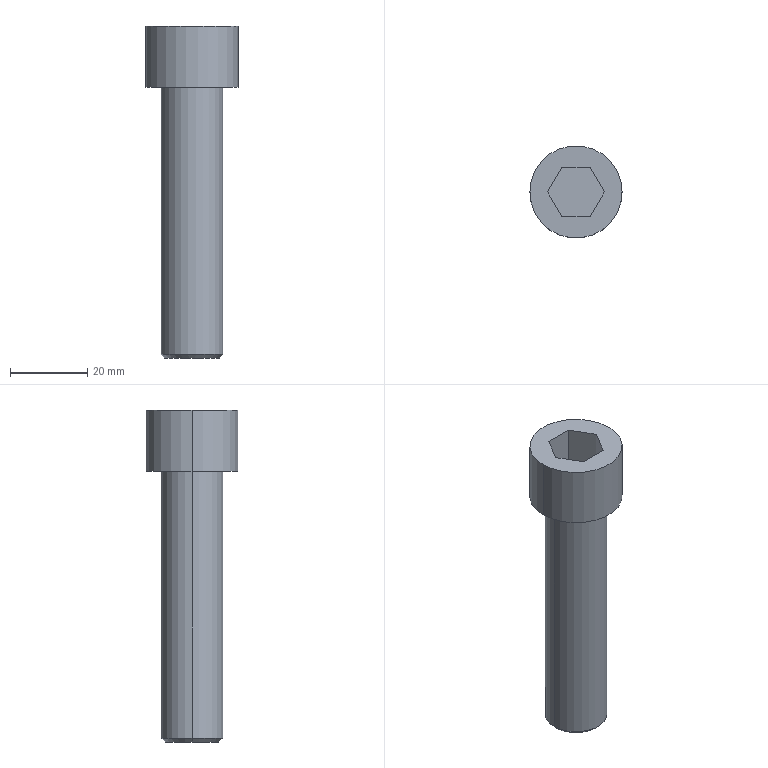Part | STEP file | 4-20.sldasm-Part-102 | 1 solid | 16 faces | box 23.812 x 23.812 x 85.725 mm | volume 19411 mm3 | plane 10 | cylinder 4 | cone 2 | commonest cylinder face diameters 15.875 x2 23.812 x2
STEP:
#1=CARTESIAN_POINT('',(-51.737,-552.065,-130.4));
#2=VERTEX_POINT('',#1);
#3=CARTESIAN_POINT('',(-65.738,-552.065,-130.4));
#4=VERTEX_POINT('',#3);
#5=CARTESIAN_POINT('',(-58.738,-552.065,-130.4));
#6=DIRECTION('',(0.,0.,-1.));
#7=DIRECTION('',(-1.,0.,0.));
#8=AXIS2_PLACEMENT_3D('',#5,#6,#7);
#9=CIRCLE('',#8,7.);
#10=EDGE_CURVE('',#2,#4,#9,.T.);
#11=ORIENTED_EDGE('',*,*,#10,.F.);
#12=CARTESIAN_POINT('',(-50.8,-552.065,-129.463));
#13=VERTEX_POINT('',#12);
#14=CARTESIAN_POINT('',(-50.8,-552.065,-129.463));
#15=DIRECTION('',(0.7071,0.,0.7071));
#16=VECTOR('',#15,1000.);
#17=LINE('',#14,#16);
#18=EDGE_CURVE('',#2,#13,#17,.T.);
#19=ORIENTED_EDGE('',*,*,#18,.T.);
#20=CARTESIAN_POINT('',(-66.675,-552.065,-129.463));
#21=VERTEX_POINT('',#20);
#22=CARTESIAN_POINT('',(-58.738,-552.065,-129.463));
#23=DIRECTION('',(0.,0.,1.));
#24=DIRECTION('',(-1.,0.,0.));
#25=AXIS2_PLACEMENT_3D('',#22,#23,#24);
#26=CIRCLE('',#25,7.937);
#27=EDGE_CURVE('',#21,#13,#26,.T.);
#28=ORIENTED_EDGE('',*,*,#27,.F.);
#29=CARTESIAN_POINT('',(-66.675,-552.065,-129.463));
#30=DIRECTION('',(-0.7071,0.,0.7071));
#31=VECTOR('',#30,1000.);
#32=LINE('',#29,#31);
#33=EDGE_CURVE('',#4,#21,#32,.T.);
#34=ORIENTED_EDGE('',*,*,#33,.F.);
#35=EDGE_LOOP('',(#11,#19,#28,#34));
#36=FACE_OUTER_BOUND('',#35,.T.);
#37=CARTESIAN_POINT('',(-58.738,-552.065,-129.463));
#38=DIRECTION('',(0.,0.,1.));
#39=DIRECTION('',(-1.,0.,0.));
#40=AXIS2_PLACEMENT_3D('',#37,#38,#39);
#41=CONICAL_SURFACE('',#40,7.937,0.7854);
#42=ADVANCED_FACE('',(#36),#41,.T.);
#43=CARTESIAN_POINT('',(-70.644,-552.065,-60.55));
#44=VERTEX_POINT('',#43);
#45=CARTESIAN_POINT('',(-46.831,-552.065,-60.55));
#46=VERTEX_POINT('',#45);
#47=CARTESIAN_POINT('',(-58.738,-552.065,-60.55));
#48=DIRECTION('',(0.,0.,1.));
#49=DIRECTION('',(-1.,0.,0.));
#50=AXIS2_PLACEMENT_3D('',#47,#48,#49);
#51=CIRCLE('',#50,11.906);
#52=EDGE_CURVE('',#44,#46,#51,.T.);
#53=ORIENTED_EDGE('',*,*,#52,.T.);
#54=CARTESIAN_POINT('',(-46.831,-552.065,-44.675));
#55=VERTEX_POINT('',#54);
#56=CARTESIAN_POINT('',(-46.831,-552.065,-60.55));
#57=DIRECTION('',(0.,0.,1.));
#58=VECTOR('',#57,1000.);
#59=LINE('',#56,#58);
#60=EDGE_CURVE('',#46,#55,#59,.T.);
#61=ORIENTED_EDGE('',*,*,#60,.T.);
#62=CARTESIAN_POINT('',(-70.644,-552.065,-44.675));
#63=VERTEX_POINT('',#62);
#64=CARTESIAN_POINT('',(-58.738,-552.065,-44.675));
#65=DIRECTION('',(0.,0.,1.));
#66=DIRECTION('',(-1.,0.,0.));
#67=AXIS2_PLACEMENT_3D('',#64,#65,#66);
#68=CIRCLE('',#67,11.906);
#69=EDGE_CURVE('',#63,#55,#68,.T.);
#70=ORIENTED_EDGE('',*,*,#69,.F.);
#71=CARTESIAN_POINT('',(-70.644,-552.065,-60.55));
#72=DIRECTION('',(0.,0.,1.));
#73=VECTOR('',#72,1000.);
#74=LINE('',#71,#73);
#75=EDGE_CURVE('',#44,#63,#74,.T.);
#76=ORIENTED_EDGE('',*,*,#75,.F.);
#77=EDGE_LOOP('',(#53,#61,#70,#76));
#78=FACE_OUTER_BOUND('',#77,.T.);
#79=CARTESIAN_POINT('',(-58.738,-552.065,-60.55));
#80=DIRECTION('',(0.,0.,1.));
#81=DIRECTION('',(-1.,0.,0.));
#82=AXIS2_PLACEMENT_3D('',#79,#80,#81);
#83=CYLINDRICAL_SURFACE('',#82,11.906);
#84=ADVANCED_FACE('',(#78),#83,.T.);
#85=CARTESIAN_POINT('',(-66.675,-552.065,-60.55));
#86=VERTEX_POINT('',#85);
#87=CARTESIAN_POINT('',(-50.8,-552.065,-60.55));
#88=VERTEX_POINT('',#87);
#89=CARTESIAN_POINT('',(-58.738,-552.065,-60.55));
#90=DIRECTION('',(0.,0.,1.));
#91=DIRECTION('',(-1.,0.,0.));
#92=AXIS2_PLACEMENT_3D('',#89,#90,#91);
#93=CIRCLE('',#92,7.937);
#94=EDGE_CURVE('',#86,#88,#93,.T.);
#95=ORIENTED_EDGE('',*,*,#94,.F.);
#96=CARTESIAN_POINT('',(-66.675,-552.065,-60.55));
#97=DIRECTION('',(0.,0.,-1.));
#98=VECTOR('',#97,1000.);
#99=LINE('',#96,#98);
#100=EDGE_CURVE('',#86,#21,#99,.T.);
#101=ORIENTED_EDGE('',*,*,#100,.T.);
#102=ORIENTED_EDGE('',*,*,#27,.T.);
#103=CARTESIAN_POINT('',(-50.8,-552.065,-60.55));
#104=DIRECTION('',(0.,0.,-1.));
#105=VECTOR('',#104,1000.);
#106=LINE('',#103,#105);
#107=EDGE_CURVE('',#88,#13,#106,.T.);
#108=ORIENTED_EDGE('',*,*,#107,.F.);
#109=EDGE_LOOP('',(#95,#101,#102,#108));
#110=FACE_OUTER_BOUND('',#109,.T.);
#111=CARTESIAN_POINT('',(-58.738,-552.065,-60.55));
#112=DIRECTION('',(0.,0.,-1.));
#113=DIRECTION('',(1.,0.,0.));
#114=AXIS2_PLACEMENT_3D('',#111,#112,#113);
#115=CYLINDRICAL_SURFACE('',#114,7.938);
#116=ADVANCED_FACE('',(#110),#115,.T.);
#117=ORIENTED_EDGE('',*,*,#100,.F.);
#118=CARTESIAN_POINT('',(-58.738,-552.065,-60.55));
#119=DIRECTION('',(0.,0.,1.));
#120=DIRECTION('',(-1.,0.,0.));
#121=AXIS2_PLACEMENT_3D('',#118,#119,#120);
#122=CIRCLE('',#121,7.937);
#123=EDGE_CURVE('',#88,#86,#122,.T.);
#124=ORIENTED_EDGE('',*,*,#123,.F.);
#125=ORIENTED_EDGE('',*,*,#107,.T.);
#126=CARTESIAN_POINT('',(-58.738,-552.065,-129.463));
#127=DIRECTION('',(0.,0.,1.));
#128=DIRECTION('',(-1.,0.,0.));
#129=AXIS2_PLACEMENT_3D('',#126,#127,#128);
#130=CIRCLE('',#129,7.937);
#131=EDGE_CURVE('',#13,#21,#130,.T.);
#132=ORIENTED_EDGE('',*,*,#131,.T.);
#133=EDGE_LOOP('',(#117,#124,#125,#132));
#134=FACE_OUTER_BOUND('',#133,.T.);
#135=CARTESIAN_POINT('',(-58.738,-552.065,-60.55));
#136=DIRECTION('',(0.,0.,-1.));
#137=DIRECTION('',(1.,0.,0.));
#138=AXIS2_PLACEMENT_3D('',#135,#136,#137);
#139=CYLINDRICAL_SURFACE('',#138,7.938);
#140=ADVANCED_FACE('',(#134),#139,.T.);
#141=CARTESIAN_POINT('',(-58.738,-552.065,-130.4));
#142=DIRECTION('',(0.,0.,-1.));
#143=DIRECTION('',(-1.,0.,0.));
#144=AXIS2_PLACEMENT_3D('',#141,#142,#143);
#145=CIRCLE('',#144,7.);
#146=EDGE_CURVE('',#4,#2,#145,.T.);
#147=ORIENTED_EDGE('',*,*,#146,.T.);
#148=ORIENTED_EDGE('',*,*,#10,.T.);
#149=EDGE_LOOP('',(#147,#148));
#150=FACE_OUTER_BOUND('',#149,.T.);
#151=CARTESIAN_POINT('',(-58.738,-552.065,-130.4));
#152=DIRECTION('',(0.,0.,1.));
#153=DIRECTION('',(-1.,0.,0.));
#154=AXIS2_PLACEMENT_3D('',#151,#152,#153);
#155=PLANE('',#154);
#156=ADVANCED_FACE('',(#150),#155,.F.);
#157=ORIENTED_EDGE('',*,*,#52,.F.);
#158=CARTESIAN_POINT('',(-58.738,-552.065,-60.55));
#159=DIRECTION('',(0.,0.,1.));
#160=DIRECTION('',(-1.,0.,0.));
#161=AXIS2_PLACEMENT_3D('',#158,#159,#160);
#162=CIRCLE('',#161,11.906);
#163=EDGE_CURVE('',#46,#44,#162,.T.);
#164=ORIENTED_EDGE('',*,*,#163,.F.);
#165=EDGE_LOOP('',(#157,#164));
#166=FACE_OUTER_BOUND('',#165,.T.);
#167=ORIENTED_EDGE('',*,*,#123,.T.);
#168=ORIENTED_EDGE('',*,*,#94,.T.);
#169=EDGE_LOOP('',(#167,#168));
#170=FACE_BOUND('',#169,.T.);
#171=CARTESIAN_POINT('',(-58.738,-552.065,-60.55));
#172=DIRECTION('',(0.,0.,-1.));
#173=DIRECTION('',(1.,0.,0.));
#174=AXIS2_PLACEMENT_3D('',#171,#172,#173);
#175=PLANE('',#174);
#176=ADVANCED_FACE('',(#166,#170),#175,.T.);
#177=CARTESIAN_POINT('',(-55.071,-545.715,-44.675));
#178=VERTEX_POINT('',#177);
#179=CARTESIAN_POINT('',(-62.404,-545.715,-44.675));
#180=VERTEX_POINT('',#179);
#181=CARTESIAN_POINT('',(-55.071,-545.715,-44.675));
#182=DIRECTION('',(-1.,0.,0.));
#183=VECTOR('',#182,1000.);
#184=LINE('',#181,#183);
#185=EDGE_CURVE('',#178,#180,#184,.T.);
#186=ORIENTED_EDGE('',*,*,#185,.F.);
#187=CARTESIAN_POINT('',(-51.405,-552.065,-44.675));
#188=VERTEX_POINT('',#187);
#189=CARTESIAN_POINT('',(-51.405,-552.065,-44.675));
#190=DIRECTION('',(-0.5,0.866,0.));
#191=VECTOR('',#190,1000.);
#192=LINE('',#189,#191);
#193=EDGE_CURVE('',#188,#178,#192,.T.);
#194=ORIENTED_EDGE('',*,*,#193,.F.);
#195=CARTESIAN_POINT('',(-55.071,-558.415,-44.675));
#196=VERTEX_POINT('',#195);
#197=CARTESIAN_POINT('',(-55.071,-558.415,-44.675));
#198=DIRECTION('',(0.5,0.866,0.));
#199=VECTOR('',#198,1000.);
#200=LINE('',#197,#199);
#201=EDGE_CURVE('',#196,#188,#200,.T.);
#202=ORIENTED_EDGE('',*,*,#201,.F.);
#203=CARTESIAN_POINT('',(-62.404,-558.415,-44.675));
#204=VERTEX_POINT('',#203);
#205=CARTESIAN_POINT('',(-62.404,-558.415,-44.675));
#206=DIRECTION('',(1.,0.,0.));
#207=VECTOR('',#206,1000.);
#208=LINE('',#205,#207);
#209=EDGE_CURVE('',#204,#196,#208,.T.);
#210=ORIENTED_EDGE('',*,*,#209,.F.);
#211=CARTESIAN_POINT('',(-66.07,-552.065,-44.675));
#212=VERTEX_POINT('',#211);
#213=CARTESIAN_POINT('',(-66.07,-552.065,-44.675));
#214=DIRECTION('',(0.5,-0.866,0.));
#215=VECTOR('',#214,1000.);
#216=LINE('',#213,#215);
#217=EDGE_CURVE('',#212,#204,#216,.T.);
#218=ORIENTED_EDGE('',*,*,#217,.F.);
#219=CARTESIAN_POINT('',(-62.404,-545.715,-44.675));
#220=DIRECTION('',(-0.5,-0.866,0.));
#221=VECTOR('',#220,1000.);
#222=LINE('',#219,#221);
#223=EDGE_CURVE('',#180,#212,#222,.T.);
#224=ORIENTED_EDGE('',*,*,#223,.F.);
#225=EDGE_LOOP('',(#186,#194,#202,#210,#218,#224));
#226=FACE_BOUND('',#225,.T.);
#227=ORIENTED_EDGE('',*,*,#69,.T.);
#228=CARTESIAN_POINT('',(-58.738,-552.065,-44.675));
#229=DIRECTION('',(0.,0.,1.));
#230=DIRECTION('',(-1.,0.,0.));
#231=AXIS2_PLACEMENT_3D('',#228,#229,#230);
#232=CIRCLE('',#231,11.906);
#233=EDGE_CURVE('',#55,#63,#232,.T.);
#234=ORIENTED_EDGE('',*,*,#233,.T.);
#235=EDGE_LOOP('',(#227,#234));
#236=FACE_OUTER_BOUND('',#235,.T.);
#237=CARTESIAN_POINT('',(-58.738,-552.065,-44.675));
#238=DIRECTION('',(0.,0.,1.));
#239=DIRECTION('',(-1.,0.,0.));
#240=AXIS2_PLACEMENT_3D('',#237,#238,#239);
#241=PLANE('',#240);
#242=ADVANCED_FACE('',(#226,#236),#241,.T.);
#243=ORIENTED_EDGE('',*,*,#60,.F.);
#244=ORIENTED_EDGE('',*,*,#163,.T.);
#245=ORIENTED_EDGE('',*,*,#75,.T.);
#246=ORIENTED_EDGE('',*,*,#233,.F.);
#247=EDGE_LOOP('',(#243,#244,#245,#246));
#248=FACE_OUTER_BOUND('',#247,.T.);
#249=CARTESIAN_POINT('',(-58.738,-552.065,-60.55));
#250=DIRECTION('',(0.,0.,1.));
#251=DIRECTION('',(-1.,0.,0.));
#252=AXIS2_PLACEMENT_3D('',#249,#250,#251);
#253=CYLINDRICAL_SURFACE('',#252,11.906);
#254=ADVANCED_FACE('',(#248),#253,.T.);
#255=ORIENTED_EDGE('',*,*,#18,.F.);
#256=ORIENTED_EDGE('',*,*,#146,.F.);
#257=ORIENTED_EDGE('',*,*,#33,.T.);
#258=ORIENTED_EDGE('',*,*,#131,.F.);
#259=EDGE_LOOP('',(#255,#256,#257,#258));
#260=FACE_OUTER_BOUND('',#259,.T.);
#261=CARTESIAN_POINT('',(-58.738,-552.065,-129.463));
#262=DIRECTION('',(0.,0.,1.));
#263=DIRECTION('',(-1.,0.,0.));
#264=AXIS2_PLACEMENT_3D('',#261,#262,#263);
#265=CONICAL_SURFACE('',#264,7.937,0.7854);
#266=ADVANCED_FACE('',(#260),#265,.T.);
#267=ORIENTED_EDGE('',*,*,#185,.T.);
#268=CARTESIAN_POINT('',(-62.404,-545.715,-55.153));
#269=VERTEX_POINT('',#268);
#270=CARTESIAN_POINT('',(-62.404,-545.715,-55.153));
#271=DIRECTION('',(0.,0.,1.));
#272=VECTOR('',#271,1000.);
#273=LINE('',#270,#272);
#274=EDGE_CURVE('',#269,#180,#273,.T.);
#275=ORIENTED_EDGE('',*,*,#274,.F.);
#276=CARTESIAN_POINT('',(-55.071,-545.715,-55.153));
#277=VERTEX_POINT('',#276);
#278=CARTESIAN_POINT('',(-55.071,-545.715,-55.153));
#279=DIRECTION('',(-1.,0.,0.));
#280=VECTOR('',#279,1000.);
#281=LINE('',#278,#280);
#282=EDGE_CURVE('',#277,#269,#281,.T.);
#283=ORIENTED_EDGE('',*,*,#282,.F.);
#284=CARTESIAN_POINT('',(-55.071,-545.715,-55.153));
#285=DIRECTION('',(0.,0.,1.));
#286=VECTOR('',#285,1000.);
#287=LINE('',#284,#286);
#288=EDGE_CURVE('',#277,#178,#287,.T.);
#289=ORIENTED_EDGE('',*,*,#288,.T.);
#290=EDGE_LOOP('',(#267,#275,#283,#289));
#291=FACE_OUTER_BOUND('',#290,.T.);
#292=CARTESIAN_POINT('',(-55.071,-545.715,-55.153));
#293=DIRECTION('',(0.,1.,0.));
#294=DIRECTION('',(0.,0.,-1.));
#295=AXIS2_PLACEMENT_3D('',#292,#293,#294);
#296=PLANE('',#295);
#297=ADVANCED_FACE('',(#291),#296,.F.);
#298=ORIENTED_EDGE('',*,*,#223,.T.);
#299=CARTESIAN_POINT('',(-66.07,-552.065,-55.153));
#300=VERTEX_POINT('',#299);
#301=CARTESIAN_POINT('',(-66.07,-552.065,-55.153));
#302=DIRECTION('',(0.,0.,1.));
#303=VECTOR('',#302,1000.);
#304=LINE('',#301,#303);
#305=EDGE_CURVE('',#300,#212,#304,.T.);
#306=ORIENTED_EDGE('',*,*,#305,.F.);
#307=CARTESIAN_POINT('',(-62.404,-545.715,-55.153));
#308=DIRECTION('',(-0.5,-0.866,0.));
#309=VECTOR('',#308,1000.);
#310=LINE('',#307,#309);
#311=EDGE_CURVE('',#269,#300,#310,.T.);
#312=ORIENTED_EDGE('',*,*,#311,.F.);
#313=ORIENTED_EDGE('',*,*,#274,.T.);
#314=EDGE_LOOP('',(#298,#306,#312,#313));
#315=FACE_OUTER_BOUND('',#314,.T.);
#316=CARTESIAN_POINT('',(-62.404,-545.715,-55.153));
#317=DIRECTION('',(-0.866,0.5,0.));
#318=DIRECTION('',(-0.5,-0.866,0.));
#319=AXIS2_PLACEMENT_3D('',#316,#317,#318);
#320=PLANE('',#319);
#321=ADVANCED_FACE('',(#315),#320,.F.);
#322=ORIENTED_EDGE('',*,*,#217,.T.);
#323=CARTESIAN_POINT('',(-62.404,-558.415,-55.153));
#324=VERTEX_POINT('',#323);
#325=CARTESIAN_POINT('',(-62.404,-558.415,-55.153));
#326=DIRECTION('',(0.,0.,1.));
#327=VECTOR('',#326,1000.);
#328=LINE('',#325,#327);
#329=EDGE_CURVE('',#324,#204,#328,.T.);
#330=ORIENTED_EDGE('',*,*,#329,.F.);
#331=CARTESIAN_POINT('',(-66.07,-552.065,-55.153));
#332=DIRECTION('',(0.5,-0.866,0.));
#333=VECTOR('',#332,1000.);
#334=LINE('',#331,#333);
#335=EDGE_CURVE('',#300,#324,#334,.T.);
#336=ORIENTED_EDGE('',*,*,#335,.F.);
#337=ORIENTED_EDGE('',*,*,#305,.T.);
#338=EDGE_LOOP('',(#322,#330,#336,#337));
#339=FACE_OUTER_BOUND('',#338,.T.);
#340=CARTESIAN_POINT('',(-66.07,-552.065,-55.153));
#341=DIRECTION('',(-0.866,-0.5,0.));
#342=DIRECTION('',(0.5,-0.866,0.));
#343=AXIS2_PLACEMENT_3D('',#340,#341,#342);
#344=PLANE('',#343);
#345=ADVANCED_FACE('',(#339),#344,.F.);
#346=ORIENTED_EDGE('',*,*,#209,.T.);
#347=CARTESIAN_POINT('',(-55.071,-558.415,-55.153));
#348=VERTEX_POINT('',#347);
#349=CARTESIAN_POINT('',(-55.071,-558.415,-55.153));
#350=DIRECTION('',(0.,0.,1.));
#351=VECTOR('',#350,1000.);
#352=LINE('',#349,#351);
#353=EDGE_CURVE('',#348,#196,#352,.T.);
#354=ORIENTED_EDGE('',*,*,#353,.F.);
#355=CARTESIAN_POINT('',(-62.404,-558.415,-55.153));
#356=DIRECTION('',(1.,0.,0.));
#357=VECTOR('',#356,1000.);
#358=LINE('',#355,#357);
#359=EDGE_CURVE('',#324,#348,#358,.T.);
#360=ORIENTED_EDGE('',*,*,#359,.F.);
#361=ORIENTED_EDGE('',*,*,#329,.T.);
#362=EDGE_LOOP('',(#346,#354,#360,#361));
#363=FACE_OUTER_BOUND('',#362,.T.);
#364=CARTESIAN_POINT('',(-62.404,-558.415,-55.153));
#365=DIRECTION('',(0.,-1.,0.));
#366=DIRECTION('',(0.,0.,1.));
#367=AXIS2_PLACEMENT_3D('',#364,#365,#366);
#368=PLANE('',#367);
#369=ADVANCED_FACE('',(#363),#368,.F.);
#370=ORIENTED_EDGE('',*,*,#201,.T.);
#371=CARTESIAN_POINT('',(-51.405,-552.065,-55.153));
#372=VERTEX_POINT('',#371);
#373=CARTESIAN_POINT('',(-51.405,-552.065,-55.153));
#374=DIRECTION('',(0.,0.,1.));
#375=VECTOR('',#374,1000.);
#376=LINE('',#373,#375);
#377=EDGE_CURVE('',#372,#188,#376,.T.);
#378=ORIENTED_EDGE('',*,*,#377,.F.);
#379=CARTESIAN_POINT('',(-55.071,-558.415,-55.153));
#380=DIRECTION('',(0.5,0.866,0.));
#381=VECTOR('',#380,1000.);
#382=LINE('',#379,#381);
#383=EDGE_CURVE('',#348,#372,#382,.T.);
#384=ORIENTED_EDGE('',*,*,#383,.F.);
#385=ORIENTED_EDGE('',*,*,#353,.T.);
#386=EDGE_LOOP('',(#370,#378,#384,#385));
#387=FACE_OUTER_BOUND('',#386,.T.);
#388=CARTESIAN_POINT('',(-55.071,-558.415,-55.153));
#389=DIRECTION('',(0.866,-0.5,0.));
#390=DIRECTION('',(0.5,0.866,0.));
#391=AXIS2_PLACEMENT_3D('',#388,#389,#390);
#392=PLANE('',#391);
#393=ADVANCED_FACE('',(#387),#392,.F.);
#394=ORIENTED_EDGE('',*,*,#193,.T.);
#395=ORIENTED_EDGE('',*,*,#288,.F.);
#396=CARTESIAN_POINT('',(-51.405,-552.065,-55.153));
#397=DIRECTION('',(-0.5,0.866,0.));
#398=VECTOR('',#397,1000.);
#399=LINE('',#396,#398);
#400=EDGE_CURVE('',#372,#277,#399,.T.);
#401=ORIENTED_EDGE('',*,*,#400,.F.);
#402=ORIENTED_EDGE('',*,*,#377,.T.);
#403=EDGE_LOOP('',(#394,#395,#401,#402));
#404=FACE_OUTER_BOUND('',#403,.T.);
#405=CARTESIAN_POINT('',(-51.405,-552.065,-55.153));
#406=DIRECTION('',(0.866,0.5,0.));
#407=DIRECTION('',(-0.5,0.866,0.));
#408=AXIS2_PLACEMENT_3D('',#405,#406,#407);
#409=PLANE('',#408);
#410=ADVANCED_FACE('',(#404),#409,.F.);
#411=ORIENTED_EDGE('',*,*,#282,.T.);
#412=ORIENTED_EDGE('',*,*,#311,.T.);
#413=ORIENTED_EDGE('',*,*,#335,.T.);
#414=ORIENTED_EDGE('',*,*,#359,.T.);
#415=ORIENTED_EDGE('',*,*,#383,.T.);
#416=ORIENTED_EDGE('',*,*,#400,.T.);
#417=EDGE_LOOP('',(#411,#412,#413,#414,#415,#416));
#418=FACE_OUTER_BOUND('',#417,.T.);
#419=CARTESIAN_POINT('',(-62.404,-545.715,-55.153));
#420=DIRECTION('',(0.,0.,1.));
#421=DIRECTION('',(-1.,0.,0.));
#422=AXIS2_PLACEMENT_3D('',#419,#420,#421);
#423=PLANE('',#422);
#424=ADVANCED_FACE('',(#418),#423,.T.);
#425=CLOSED_SHELL('',(#42,#84,#116,#140,#156,#176,#242,#254,#266,#297,#321,#345,#369,#393,#410,#424));
#426=MANIFOLD_SOLID_BREP('',#425);
#427=CARTESIAN_POINT('',(0.,0.,0.));
#428=DIRECTION('',(0.,0.,1.));
#429=DIRECTION('',(1.,0.,0.));
#430=AXIS2_PLACEMENT_3D('',#427,#428,#429);
#431=(LENGTH_UNIT()NAMED_UNIT(*)SI_UNIT(.MILLI.,.METRE.));
#432=UNCERTAINTY_MEASURE_WITH_UNIT(LENGTH_MEASURE(0.00001),#431,'','');
#433=(NAMED_UNIT(*)PLANE_ANGLE_UNIT()SI_UNIT($,.RADIAN.));
#434=(NAMED_UNIT(*)SI_UNIT($,.STERADIAN.)SOLID_ANGLE_UNIT());
#435=(GEOMETRIC_REPRESENTATION_CONTEXT(3)GLOBAL_UNCERTAINTY_ASSIGNED_CONTEXT((#432))GLOBAL_UNIT_ASSIGNED_CONTEXT((#431,#433,#434))REPRESENTATION_CONTEXT('',''));
#436=ADVANCED_BREP_SHAPE_REPRESENTATION('',(#426,#430),#435);